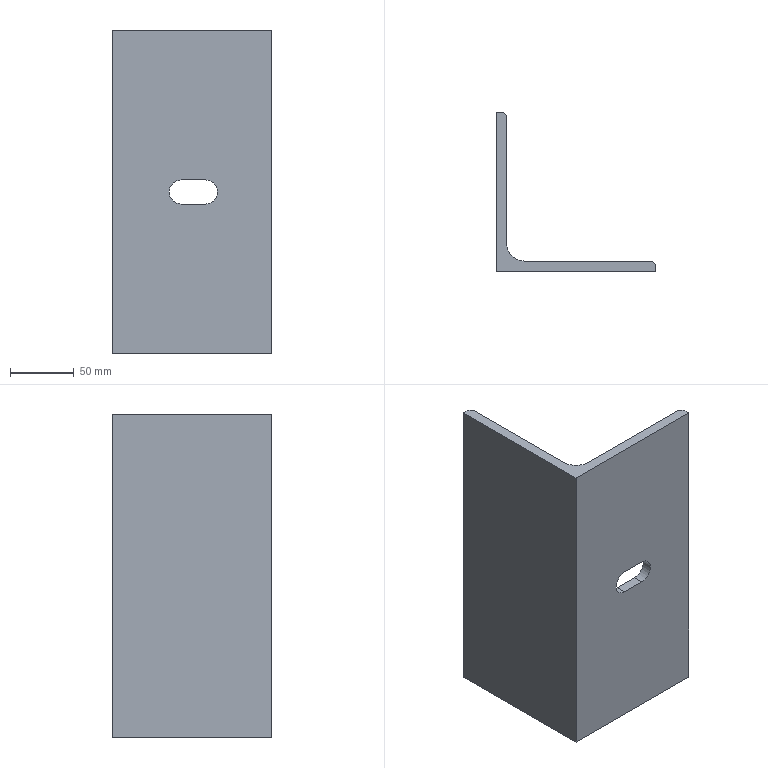Part | SolidWorks | features Extrusion 1, ICE 1 | 1 solid | 15 faces | box 125 x 125 x 254 mm | volume 495500 mm3 | plane 10 | cylinder 5 | commonest cylinder face diameters 8 x2 19.05 x2 28 x1
STEP:
#1=CARTESIAN_POINT('',(4.,125.,-127.));
#2=VERTEX_POINT('',#1);
#3=CARTESIAN_POINT('',(0.,125.,-127.));
#4=VERTEX_POINT('',#3);
#5=CARTESIAN_POINT('',(0.,125.,-127.));
#6=DIRECTION('',(-1.,0.,0.));
#7=VECTOR('',#6,1000.);
#8=LINE('',#5,#7);
#9=EDGE_CURVE('',#2,#4,#8,.T.);
#10=ORIENTED_EDGE('',*,*,#9,.T.);
#11=CARTESIAN_POINT('',(0.,125.,127.));
#12=VERTEX_POINT('',#11);
#13=CARTESIAN_POINT('',(0.,125.,127.));
#14=DIRECTION('',(0.,0.,-1.));
#15=VECTOR('',#14,1000.);
#16=LINE('',#13,#15);
#17=EDGE_CURVE('',#12,#4,#16,.T.);
#18=ORIENTED_EDGE('',*,*,#17,.F.);
#19=CARTESIAN_POINT('',(4.,125.,127.));
#20=VERTEX_POINT('',#19);
#21=CARTESIAN_POINT('',(0.,125.,127.));
#22=DIRECTION('',(-1.,0.,0.));
#23=VECTOR('',#22,1000.);
#24=LINE('',#21,#23);
#25=EDGE_CURVE('',#20,#12,#24,.T.);
#26=ORIENTED_EDGE('',*,*,#25,.F.);
#27=CARTESIAN_POINT('',(4.,125.,127.));
#28=DIRECTION('',(0.,0.,-1.));
#29=VECTOR('',#28,1000.);
#30=LINE('',#27,#29);
#31=EDGE_CURVE('',#20,#2,#30,.T.);
#32=ORIENTED_EDGE('',*,*,#31,.T.);
#33=EDGE_LOOP('',(#10,#18,#26,#32));
#34=FACE_OUTER_BOUND('',#33,.T.);
#35=CARTESIAN_POINT('',(0.,125.,127.));
#36=DIRECTION('',(0.,-1.,0.));
#37=DIRECTION('',(0.,0.,-1.));
#38=AXIS2_PLACEMENT_3D('',#35,#36,#37);
#39=PLANE('',#38);
#40=ADVANCED_FACE('',(#34),#39,.F.);
#41=CARTESIAN_POINT('',(0.,0.,-127.));
#42=VERTEX_POINT('',#41);
#43=CARTESIAN_POINT('',(0.,125.,-127.));
#44=DIRECTION('',(0.,-1.,0.));
#45=VECTOR('',#44,1000.);
#46=LINE('',#43,#45);
#47=EDGE_CURVE('',#4,#42,#46,.T.);
#48=ORIENTED_EDGE('',*,*,#47,.T.);
#49=CARTESIAN_POINT('',(0.,0.,127.));
#50=VERTEX_POINT('',#49);
#51=CARTESIAN_POINT('',(0.,0.,127.));
#52=DIRECTION('',(0.,0.,-1.));
#53=VECTOR('',#52,1000.);
#54=LINE('',#51,#53);
#55=EDGE_CURVE('',#50,#42,#54,.T.);
#56=ORIENTED_EDGE('',*,*,#55,.F.);
#57=CARTESIAN_POINT('',(0.,125.,127.));
#58=DIRECTION('',(0.,-1.,0.));
#59=VECTOR('',#58,1000.);
#60=LINE('',#57,#59);
#61=EDGE_CURVE('',#12,#50,#60,.T.);
#62=ORIENTED_EDGE('',*,*,#61,.F.);
#63=ORIENTED_EDGE('',*,*,#17,.T.);
#64=EDGE_LOOP('',(#48,#56,#62,#63));
#65=FACE_OUTER_BOUND('',#64,.T.);
#66=CARTESIAN_POINT('',(0.,125.,127.));
#67=DIRECTION('',(1.,0.,0.));
#68=DIRECTION('',(0.,1.,0.));
#69=AXIS2_PLACEMENT_3D('',#66,#67,#68);
#70=PLANE('',#69);
#71=ADVANCED_FACE('',(#65),#70,.F.);
#72=CARTESIAN_POINT('',(73.025,0.,-9.525));
#73=VERTEX_POINT('',#72);
#74=CARTESIAN_POINT('',(53.975,0.,-9.525));
#75=VERTEX_POINT('',#74);
#76=CARTESIAN_POINT('',(0.,0.,-9.525));
#77=DIRECTION('',(-1.,0.,0.));
#78=VECTOR('',#77,1000.);
#79=LINE('',#76,#78);
#80=EDGE_CURVE('',#73,#75,#79,.T.);
#81=ORIENTED_EDGE('',*,*,#80,.T.);
#82=CARTESIAN_POINT('',(53.975,0.,9.525));
#83=VERTEX_POINT('',#82);
#84=CARTESIAN_POINT('',(53.975,0.,0.));
#85=DIRECTION('',(0.,1.,0.));
#86=DIRECTION('',(0.,0.,1.));
#87=AXIS2_PLACEMENT_3D('',#84,#85,#86);
#88=CIRCLE('',#87,9.525);
#89=EDGE_CURVE('',#75,#83,#88,.T.);
#90=ORIENTED_EDGE('',*,*,#89,.T.);
#91=CARTESIAN_POINT('',(73.025,0.,9.525));
#92=VERTEX_POINT('',#91);
#93=CARTESIAN_POINT('',(0.,0.,9.525));
#94=DIRECTION('',(1.,0.,0.));
#95=VECTOR('',#94,1000.);
#96=LINE('',#93,#95);
#97=EDGE_CURVE('',#83,#92,#96,.T.);
#98=ORIENTED_EDGE('',*,*,#97,.T.);
#99=CARTESIAN_POINT('',(73.025,0.,0.));
#100=DIRECTION('',(0.,1.,0.));
#101=DIRECTION('',(0.,0.,1.));
#102=AXIS2_PLACEMENT_3D('',#99,#100,#101);
#103=CIRCLE('',#102,9.525);
#104=EDGE_CURVE('',#92,#73,#103,.T.);
#105=ORIENTED_EDGE('',*,*,#104,.T.);
#106=EDGE_LOOP('',(#81,#90,#98,#105));
#107=FACE_BOUND('',#106,.T.);
#108=CARTESIAN_POINT('',(125.,0.,-127.));
#109=VERTEX_POINT('',#108);
#110=CARTESIAN_POINT('',(0.,0.,-127.));
#111=DIRECTION('',(1.,0.,0.));
#112=VECTOR('',#111,1000.);
#113=LINE('',#110,#112);
#114=EDGE_CURVE('',#42,#109,#113,.T.);
#115=ORIENTED_EDGE('',*,*,#114,.T.);
#116=CARTESIAN_POINT('',(125.,0.,127.));
#117=VERTEX_POINT('',#116);
#118=CARTESIAN_POINT('',(125.,0.,127.));
#119=DIRECTION('',(0.,0.,-1.));
#120=VECTOR('',#119,1000.);
#121=LINE('',#118,#120);
#122=EDGE_CURVE('',#117,#109,#121,.T.);
#123=ORIENTED_EDGE('',*,*,#122,.F.);
#124=CARTESIAN_POINT('',(0.,0.,127.));
#125=DIRECTION('',(1.,0.,0.));
#126=VECTOR('',#125,1000.);
#127=LINE('',#124,#126);
#128=EDGE_CURVE('',#50,#117,#127,.T.);
#129=ORIENTED_EDGE('',*,*,#128,.F.);
#130=ORIENTED_EDGE('',*,*,#55,.T.);
#131=EDGE_LOOP('',(#115,#123,#129,#130));
#132=FACE_OUTER_BOUND('',#131,.T.);
#133=CARTESIAN_POINT('',(0.,0.,127.));
#134=DIRECTION('',(0.,1.,0.));
#135=DIRECTION('',(0.,0.,1.));
#136=AXIS2_PLACEMENT_3D('',#133,#134,#135);
#137=PLANE('',#136);
#138=ADVANCED_FACE('',(#107,#132),#137,.F.);
#139=CARTESIAN_POINT('',(125.,4.,-127.));
#140=VERTEX_POINT('',#139);
#141=CARTESIAN_POINT('',(125.,0.,-127.));
#142=DIRECTION('',(0.,1.,0.));
#143=VECTOR('',#142,1000.);
#144=LINE('',#141,#143);
#145=EDGE_CURVE('',#109,#140,#144,.T.);
#146=ORIENTED_EDGE('',*,*,#145,.T.);
#147=CARTESIAN_POINT('',(125.,4.,127.));
#148=VERTEX_POINT('',#147);
#149=CARTESIAN_POINT('',(125.,4.,127.));
#150=DIRECTION('',(0.,0.,-1.));
#151=VECTOR('',#150,1000.);
#152=LINE('',#149,#151);
#153=EDGE_CURVE('',#148,#140,#152,.T.);
#154=ORIENTED_EDGE('',*,*,#153,.F.);
#155=CARTESIAN_POINT('',(125.,0.,127.));
#156=DIRECTION('',(0.,1.,0.));
#157=VECTOR('',#156,1000.);
#158=LINE('',#155,#157);
#159=EDGE_CURVE('',#117,#148,#158,.T.);
#160=ORIENTED_EDGE('',*,*,#159,.F.);
#161=ORIENTED_EDGE('',*,*,#122,.T.);
#162=EDGE_LOOP('',(#146,#154,#160,#161));
#163=FACE_OUTER_BOUND('',#162,.T.);
#164=CARTESIAN_POINT('',(125.,0.,127.));
#165=DIRECTION('',(-1.,0.,0.));
#166=DIRECTION('',(0.,0.,1.));
#167=AXIS2_PLACEMENT_3D('',#164,#165,#166);
#168=PLANE('',#167);
#169=ADVANCED_FACE('',(#163),#168,.F.);
#170=CARTESIAN_POINT('',(121.,8.,-127.));
#171=VERTEX_POINT('',#170);
#172=CARTESIAN_POINT('',(121.,4.,-127.));
#173=DIRECTION('',(0.,0.,1.));
#174=DIRECTION('',(1.,0.,0.));
#175=AXIS2_PLACEMENT_3D('',#172,#173,#174);
#176=CIRCLE('',#175,4.);
#177=EDGE_CURVE('',#140,#171,#176,.T.);
#178=ORIENTED_EDGE('',*,*,#177,.T.);
#179=CARTESIAN_POINT('',(121.,8.,127.));
#180=VERTEX_POINT('',#179);
#181=CARTESIAN_POINT('',(121.,8.,127.));
#182=DIRECTION('',(0.,0.,-1.));
#183=VECTOR('',#182,1000.);
#184=LINE('',#181,#183);
#185=EDGE_CURVE('',#180,#171,#184,.T.);
#186=ORIENTED_EDGE('',*,*,#185,.F.);
#187=CARTESIAN_POINT('',(121.,4.,127.));
#188=DIRECTION('',(0.,0.,1.));
#189=DIRECTION('',(1.,0.,0.));
#190=AXIS2_PLACEMENT_3D('',#187,#188,#189);
#191=CIRCLE('',#190,4.);
#192=EDGE_CURVE('',#148,#180,#191,.T.);
#193=ORIENTED_EDGE('',*,*,#192,.F.);
#194=ORIENTED_EDGE('',*,*,#153,.T.);
#195=EDGE_LOOP('',(#178,#186,#193,#194));
#196=FACE_OUTER_BOUND('',#195,.T.);
#197=CARTESIAN_POINT('',(121.,4.,127.));
#198=DIRECTION('',(0.,0.,-1.));
#199=DIRECTION('',(-1.,0.,0.));
#200=AXIS2_PLACEMENT_3D('',#197,#198,#199);
#201=CYLINDRICAL_SURFACE('',#200,4.);
#202=ADVANCED_FACE('',(#196),#201,.T.);
#203=CARTESIAN_POINT('',(53.975,8.,9.525));
#204=VERTEX_POINT('',#203);
#205=CARTESIAN_POINT('',(73.025,8.,9.525));
#206=VERTEX_POINT('',#205);
#207=CARTESIAN_POINT('',(53.975,8.,9.525));
#208=DIRECTION('',(1.,0.,0.));
#209=VECTOR('',#208,1000.);
#210=LINE('',#207,#209);
#211=EDGE_CURVE('',#204,#206,#210,.T.);
#212=ORIENTED_EDGE('',*,*,#211,.F.);
#213=CARTESIAN_POINT('',(53.975,8.,-9.525));
#214=VERTEX_POINT('',#213);
#215=CARTESIAN_POINT('',(53.975,8.,0.));
#216=DIRECTION('',(0.,1.,0.));
#217=DIRECTION('',(0.,0.,1.));
#218=AXIS2_PLACEMENT_3D('',#215,#216,#217);
#219=CIRCLE('',#218,9.525);
#220=EDGE_CURVE('',#214,#204,#219,.T.);
#221=ORIENTED_EDGE('',*,*,#220,.F.);
#222=CARTESIAN_POINT('',(73.025,8.,-9.525));
#223=VERTEX_POINT('',#222);
#224=CARTESIAN_POINT('',(53.975,8.,-9.525));
#225=DIRECTION('',(-1.,0.,0.));
#226=VECTOR('',#225,1000.);
#227=LINE('',#224,#226);
#228=EDGE_CURVE('',#223,#214,#227,.T.);
#229=ORIENTED_EDGE('',*,*,#228,.F.);
#230=CARTESIAN_POINT('',(73.025,8.,0.));
#231=DIRECTION('',(0.,1.,0.));
#232=DIRECTION('',(0.,0.,1.));
#233=AXIS2_PLACEMENT_3D('',#230,#231,#232);
#234=CIRCLE('',#233,9.525);
#235=EDGE_CURVE('',#206,#223,#234,.T.);
#236=ORIENTED_EDGE('',*,*,#235,.F.);
#237=EDGE_LOOP('',(#212,#221,#229,#236));
#238=FACE_BOUND('',#237,.T.);
#239=CARTESIAN_POINT('',(22.,8.,-127.));
#240=VERTEX_POINT('',#239);
#241=CARTESIAN_POINT('',(22.,8.,-127.));
#242=DIRECTION('',(-1.,0.,0.));
#243=VECTOR('',#242,1000.);
#244=LINE('',#241,#243);
#245=EDGE_CURVE('',#171,#240,#244,.T.);
#246=ORIENTED_EDGE('',*,*,#245,.T.);
#247=CARTESIAN_POINT('',(22.,8.,127.));
#248=VERTEX_POINT('',#247);
#249=CARTESIAN_POINT('',(22.,8.,127.));
#250=DIRECTION('',(0.,0.,-1.));
#251=VECTOR('',#250,1000.);
#252=LINE('',#249,#251);
#253=EDGE_CURVE('',#248,#240,#252,.T.);
#254=ORIENTED_EDGE('',*,*,#253,.F.);
#255=CARTESIAN_POINT('',(22.,8.,127.));
#256=DIRECTION('',(-1.,0.,0.));
#257=VECTOR('',#256,1000.);
#258=LINE('',#255,#257);
#259=EDGE_CURVE('',#180,#248,#258,.T.);
#260=ORIENTED_EDGE('',*,*,#259,.F.);
#261=ORIENTED_EDGE('',*,*,#185,.T.);
#262=EDGE_LOOP('',(#246,#254,#260,#261));
#263=FACE_OUTER_BOUND('',#262,.T.);
#264=CARTESIAN_POINT('',(22.,8.,127.));
#265=DIRECTION('',(0.,-1.,0.));
#266=DIRECTION('',(1.,0.,0.));
#267=AXIS2_PLACEMENT_3D('',#264,#265,#266);
#268=PLANE('',#267);
#269=ADVANCED_FACE('',(#238,#263),#268,.F.);
#270=CARTESIAN_POINT('',(8.,22.,-127.));
#271=VERTEX_POINT('',#270);
#272=CARTESIAN_POINT('',(22.,22.,-127.));
#273=DIRECTION('',(0.,0.,-1.));
#274=DIRECTION('',(1.,0.,0.));
#275=AXIS2_PLACEMENT_3D('',#272,#273,#274);
#276=CIRCLE('',#275,14.);
#277=EDGE_CURVE('',#240,#271,#276,.T.);
#278=ORIENTED_EDGE('',*,*,#277,.T.);
#279=CARTESIAN_POINT('',(8.,22.,127.));
#280=VERTEX_POINT('',#279);
#281=CARTESIAN_POINT('',(8.,22.,127.));
#282=DIRECTION('',(0.,0.,-1.));
#283=VECTOR('',#282,1000.);
#284=LINE('',#281,#283);
#285=EDGE_CURVE('',#280,#271,#284,.T.);
#286=ORIENTED_EDGE('',*,*,#285,.F.);
#287=CARTESIAN_POINT('',(22.,22.,127.));
#288=DIRECTION('',(0.,0.,-1.));
#289=DIRECTION('',(1.,0.,0.));
#290=AXIS2_PLACEMENT_3D('',#287,#288,#289);
#291=CIRCLE('',#290,14.);
#292=EDGE_CURVE('',#248,#280,#291,.T.);
#293=ORIENTED_EDGE('',*,*,#292,.F.);
#294=ORIENTED_EDGE('',*,*,#253,.T.);
#295=EDGE_LOOP('',(#278,#286,#293,#294));
#296=FACE_OUTER_BOUND('',#295,.T.);
#297=CARTESIAN_POINT('',(22.,22.,127.));
#298=DIRECTION('',(0.,0.,-1.));
#299=DIRECTION('',(-1.,0.,0.));
#300=AXIS2_PLACEMENT_3D('',#297,#298,#299);
#301=CYLINDRICAL_SURFACE('',#300,14.);
#302=ADVANCED_FACE('',(#296),#301,.F.);
#303=CARTESIAN_POINT('',(8.,121.,-127.));
#304=VERTEX_POINT('',#303);
#305=CARTESIAN_POINT('',(8.,121.,-127.));
#306=DIRECTION('',(0.,1.,0.));
#307=VECTOR('',#306,1000.);
#308=LINE('',#305,#307);
#309=EDGE_CURVE('',#271,#304,#308,.T.);
#310=ORIENTED_EDGE('',*,*,#309,.T.);
#311=CARTESIAN_POINT('',(8.,121.,127.));
#312=VERTEX_POINT('',#311);
#313=CARTESIAN_POINT('',(8.,121.,127.));
#314=DIRECTION('',(0.,0.,-1.));
#315=VECTOR('',#314,1000.);
#316=LINE('',#313,#315);
#317=EDGE_CURVE('',#312,#304,#316,.T.);
#318=ORIENTED_EDGE('',*,*,#317,.F.);
#319=CARTESIAN_POINT('',(8.,121.,127.));
#320=DIRECTION('',(0.,1.,0.));
#321=VECTOR('',#320,1000.);
#322=LINE('',#319,#321);
#323=EDGE_CURVE('',#280,#312,#322,.T.);
#324=ORIENTED_EDGE('',*,*,#323,.F.);
#325=ORIENTED_EDGE('',*,*,#285,.T.);
#326=EDGE_LOOP('',(#310,#318,#324,#325));
#327=FACE_OUTER_BOUND('',#326,.T.);
#328=CARTESIAN_POINT('',(8.,121.,127.));
#329=DIRECTION('',(-1.,0.,0.));
#330=DIRECTION('',(0.,-1.,0.));
#331=AXIS2_PLACEMENT_3D('',#328,#329,#330);
#332=PLANE('',#331);
#333=ADVANCED_FACE('',(#327),#332,.F.);
#334=CARTESIAN_POINT('',(4.,121.,-127.));
#335=DIRECTION('',(0.,0.,1.));
#336=DIRECTION('',(-1.,0.,0.));
#337=AXIS2_PLACEMENT_3D('',#334,#335,#336);
#338=CIRCLE('',#337,4.);
#339=EDGE_CURVE('',#304,#2,#338,.T.);
#340=ORIENTED_EDGE('',*,*,#339,.T.);
#341=ORIENTED_EDGE('',*,*,#31,.F.);
#342=CARTESIAN_POINT('',(4.,121.,127.));
#343=DIRECTION('',(0.,0.,1.));
#344=DIRECTION('',(-1.,0.,0.));
#345=AXIS2_PLACEMENT_3D('',#342,#343,#344);
#346=CIRCLE('',#345,4.);
#347=EDGE_CURVE('',#312,#20,#346,.T.);
#348=ORIENTED_EDGE('',*,*,#347,.F.);
#349=ORIENTED_EDGE('',*,*,#317,.T.);
#350=EDGE_LOOP('',(#340,#341,#348,#349));
#351=FACE_OUTER_BOUND('',#350,.T.);
#352=CARTESIAN_POINT('',(4.,121.,127.));
#353=DIRECTION('',(0.,0.,-1.));
#354=DIRECTION('',(-1.,0.,0.));
#355=AXIS2_PLACEMENT_3D('',#352,#353,#354);
#356=CYLINDRICAL_SURFACE('',#355,4.);
#357=ADVANCED_FACE('',(#351),#356,.T.);
#358=ORIENTED_EDGE('',*,*,#25,.T.);
#359=ORIENTED_EDGE('',*,*,#61,.T.);
#360=ORIENTED_EDGE('',*,*,#128,.T.);
#361=ORIENTED_EDGE('',*,*,#159,.T.);
#362=ORIENTED_EDGE('',*,*,#192,.T.);
#363=ORIENTED_EDGE('',*,*,#259,.T.);
#364=ORIENTED_EDGE('',*,*,#292,.T.);
#365=ORIENTED_EDGE('',*,*,#323,.T.);
#366=ORIENTED_EDGE('',*,*,#347,.T.);
#367=EDGE_LOOP('',(#358,#359,#360,#361,#362,#363,#364,#365,#366));
#368=FACE_OUTER_BOUND('',#367,.T.);
#369=CARTESIAN_POINT('',(4.,121.,127.));
#370=DIRECTION('',(0.,0.,-1.));
#371=DIRECTION('',(-1.,0.,0.));
#372=AXIS2_PLACEMENT_3D('',#369,#370,#371);
#373=PLANE('',#372);
#374=ADVANCED_FACE('',(#368),#373,.F.);
#375=ORIENTED_EDGE('',*,*,#9,.F.);
#376=ORIENTED_EDGE('',*,*,#339,.F.);
#377=ORIENTED_EDGE('',*,*,#309,.F.);
#378=ORIENTED_EDGE('',*,*,#277,.F.);
#379=ORIENTED_EDGE('',*,*,#245,.F.);
#380=ORIENTED_EDGE('',*,*,#177,.F.);
#381=ORIENTED_EDGE('',*,*,#145,.F.);
#382=ORIENTED_EDGE('',*,*,#114,.F.);
#383=ORIENTED_EDGE('',*,*,#47,.F.);
#384=EDGE_LOOP('',(#375,#376,#377,#378,#379,#380,#381,#382,#383));
#385=FACE_OUTER_BOUND('',#384,.T.);
#386=CARTESIAN_POINT('',(4.,121.,-127.));
#387=DIRECTION('',(0.,0.,-1.));
#388=DIRECTION('',(-1.,0.,0.));
#389=AXIS2_PLACEMENT_3D('',#386,#387,#388);
#390=PLANE('',#389);
#391=ADVANCED_FACE('',(#385),#390,.T.);
#392=CARTESIAN_POINT('',(53.975,-296.8,-9.525));
#393=DIRECTION('',(0.,1.,0.));
#394=VECTOR('',#393,1000.);
#395=LINE('',#392,#394);
#396=EDGE_CURVE('',#75,#214,#395,.T.);
#397=ORIENTED_EDGE('',*,*,#396,.T.);
#398=ORIENTED_EDGE('',*,*,#220,.T.);
#399=CARTESIAN_POINT('',(53.975,-296.8,9.525));
#400=DIRECTION('',(0.,1.,0.));
#401=VECTOR('',#400,1000.);
#402=LINE('',#399,#401);
#403=EDGE_CURVE('',#83,#204,#402,.T.);
#404=ORIENTED_EDGE('',*,*,#403,.F.);
#405=ORIENTED_EDGE('',*,*,#89,.F.);
#406=EDGE_LOOP('',(#397,#398,#404,#405));
#407=FACE_OUTER_BOUND('',#406,.T.);
#408=CARTESIAN_POINT('',(53.975,-296.8,0.));
#409=DIRECTION('',(0.,1.,0.));
#410=DIRECTION('',(0.,0.,1.));
#411=AXIS2_PLACEMENT_3D('',#408,#409,#410);
#412=CYLINDRICAL_SURFACE('',#411,9.525);
#413=ADVANCED_FACE('',(#407),#412,.F.);
#414=CARTESIAN_POINT('',(73.025,-296.8,-9.525));
#415=DIRECTION('',(0.,1.,0.));
#416=VECTOR('',#415,1000.);
#417=LINE('',#414,#416);
#418=EDGE_CURVE('',#73,#223,#417,.T.);
#419=ORIENTED_EDGE('',*,*,#418,.T.);
#420=ORIENTED_EDGE('',*,*,#228,.T.);
#421=ORIENTED_EDGE('',*,*,#396,.F.);
#422=ORIENTED_EDGE('',*,*,#80,.F.);
#423=EDGE_LOOP('',(#419,#420,#421,#422));
#424=FACE_OUTER_BOUND('',#423,.T.);
#425=CARTESIAN_POINT('',(53.975,-296.8,-9.525));
#426=DIRECTION('',(0.,0.,-1.));
#427=DIRECTION('',(-1.,0.,0.));
#428=AXIS2_PLACEMENT_3D('',#425,#426,#427);
#429=PLANE('',#428);
#430=ADVANCED_FACE('',(#424),#429,.F.);
#431=CARTESIAN_POINT('',(73.025,-296.8,9.525));
#432=DIRECTION('',(0.,1.,0.));
#433=VECTOR('',#432,1000.);
#434=LINE('',#431,#433);
#435=EDGE_CURVE('',#92,#206,#434,.T.);
#436=ORIENTED_EDGE('',*,*,#435,.T.);
#437=ORIENTED_EDGE('',*,*,#235,.T.);
#438=ORIENTED_EDGE('',*,*,#418,.F.);
#439=ORIENTED_EDGE('',*,*,#104,.F.);
#440=EDGE_LOOP('',(#436,#437,#438,#439));
#441=FACE_OUTER_BOUND('',#440,.T.);
#442=CARTESIAN_POINT('',(73.025,-296.8,0.));
#443=DIRECTION('',(0.,1.,0.));
#444=DIRECTION('',(0.,0.,1.));
#445=AXIS2_PLACEMENT_3D('',#442,#443,#444);
#446=CYLINDRICAL_SURFACE('',#445,9.525);
#447=ADVANCED_FACE('',(#441),#446,.F.);
#448=ORIENTED_EDGE('',*,*,#403,.T.);
#449=ORIENTED_EDGE('',*,*,#211,.T.);
#450=ORIENTED_EDGE('',*,*,#435,.F.);
#451=ORIENTED_EDGE('',*,*,#97,.F.);
#452=EDGE_LOOP('',(#448,#449,#450,#451));
#453=FACE_OUTER_BOUND('',#452,.T.);
#454=CARTESIAN_POINT('',(53.975,-296.8,9.525));
#455=DIRECTION('',(0.,0.,1.));
#456=DIRECTION('',(1.,0.,0.));
#457=AXIS2_PLACEMENT_3D('',#454,#455,#456);
#458=PLANE('',#457);
#459=ADVANCED_FACE('',(#453),#458,.F.);
#460=CLOSED_SHELL('',(#40,#71,#138,#169,#202,#269,#302,#333,#357,#374,#391,#413,#430,#447,#459));
#461=MANIFOLD_SOLID_BREP('',#460);
#462=CARTESIAN_POINT('',(0.,0.,0.));
#463=DIRECTION('',(0.,0.,1.));
#464=DIRECTION('',(1.,0.,0.));
#465=AXIS2_PLACEMENT_3D('',#462,#463,#464);
#466=(LENGTH_UNIT()NAMED_UNIT(*)SI_UNIT(.MILLI.,.METRE.));
#467=UNCERTAINTY_MEASURE_WITH_UNIT(LENGTH_MEASURE(0.00001),#466,'','');
#468=(NAMED_UNIT(*)PLANE_ANGLE_UNIT()SI_UNIT($,.RADIAN.));
#469=(NAMED_UNIT(*)SI_UNIT($,.STERADIAN.)SOLID_ANGLE_UNIT());
#470=(GEOMETRIC_REPRESENTATION_CONTEXT(3)GLOBAL_UNCERTAINTY_ASSIGNED_CONTEXT((#467))GLOBAL_UNIT_ASSIGNED_CONTEXT((#466,#468,#469))REPRESENTATION_CONTEXT('',''));
#471=ADVANCED_BREP_SHAPE_REPRESENTATION('',(#461,#465),#470);